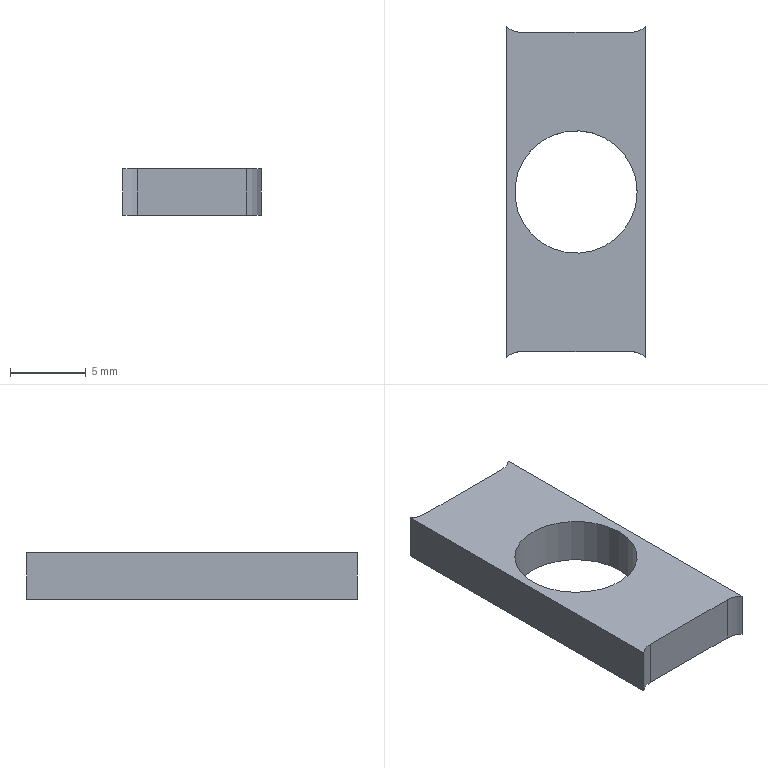Part | STEP file | 1_id370_x_t | 1 solid | 11 faces | box 9.15 x 21.764 x 3.075 mm | volume 435.444 mm3 | plane 6 | cylinder 5 | commonest cylinder face diameters 3 x4 8.06 x1
STEP:
#1=CARTESIAN_POINT('',(0.,0.,0.));
#2=DIRECTION('',(0.,0.,1.));
#3=DIRECTION('',(1.,0.,0.));
#4=AXIS2_PLACEMENT_3D('',#1,#2,#3);
#5=CARTESIAN_POINT('',(383.175,166.618,0.));
#6=VERTEX_POINT('',#5);
#7=CARTESIAN_POINT('',(382.175,167.,0.));
#8=VERTEX_POINT('',#7);
#9=CARTESIAN_POINT('',(382.175,165.5,0.));
#10=DIRECTION('',(0.,0.,1.));
#11=DIRECTION('',(1.,0.,0.));
#12=AXIS2_PLACEMENT_3D('',#9,#10,#11);
#13=CIRCLE('',#12,1.5);
#14=CARTESIAN_POINT('',(382.175,165.5,13.075));
#15=DIRECTION('',(0.,0.,-1.));
#16=DIRECTION('',(-1.,0.,0.));
#17=AXIS2_PLACEMENT_3D('',#14,#15,#16);
#18=CYLINDRICAL_SURFACE('',#17,1.5);
#19=CARTESIAN_POINT('',(3.142,13.075));
#20=DIRECTION('',(-1.,0.));
#21=VECTOR('',#20,1.);
#22=LINE('',#19,#21);
#23=(GEOMETRIC_REPRESENTATION_CONTEXT(2)PARAMETRIC_REPRESENTATION_CONTEXT()REPRESENTATION_CONTEXT('',''));
#24=DEFINITIONAL_REPRESENTATION('',(#22),#23);
#25=PCURVE('',#18,#24);
#26=CARTESIAN_POINT('',(407.126,177.154,0.));
#27=DIRECTION('',(0.,0.,1.));
#28=DIRECTION('',(0.00002249,-1.,0.));
#29=AXIS2_PLACEMENT_3D('',#26,#27,#28);
#30=PLANE('',#29);
#31=CARTESIAN_POINT('',(11.653,-24.951));
#32=DIRECTION('',(0.00002249,1.));
#33=AXIS2_PLACEMENT_2D('',#31,#32);
#34=CIRCLE('',#33,1.5);
#35=(GEOMETRIC_REPRESENTATION_CONTEXT(2)PARAMETRIC_REPRESENTATION_CONTEXT()REPRESENTATION_CONTEXT('',''));
#36=DEFINITIONAL_REPRESENTATION('',(#34),#35);
#37=PCURVE('',#30,#36);
#38=SURFACE_CURVE('',#13,(#25,#37),.PCURVE_S1.);
#39=EDGE_CURVE('',#6,#8,#38,.T.);
#40=ORIENTED_EDGE('',*,*,#39,.T.);
#41=CARTESIAN_POINT('',(382.175,167.,3.075));
#42=VERTEX_POINT('',#41);
#43=CARTESIAN_POINT('',(382.175,167.,13.075));
#44=DIRECTION('',(0.,0.,-1.));
#45=VECTOR('',#44,1.);
#46=LINE('',#43,#45);
#47=CARTESIAN_POINT('',(1.571,0.));
#48=DIRECTION('',(0.,1.));
#49=VECTOR('',#48,1.);
#50=LINE('',#47,#49);
#51=(GEOMETRIC_REPRESENTATION_CONTEXT(2)PARAMETRIC_REPRESENTATION_CONTEXT()REPRESENTATION_CONTEXT('',''));
#52=DEFINITIONAL_REPRESENTATION('',(#50),#51);
#53=PCURVE('',#18,#52);
#54=CARTESIAN_POINT('',(382.175,167.,13.075));
#55=DIRECTION('',(0.,-1.,0.));
#56=DIRECTION('',(0.,0.,-1.));
#57=AXIS2_PLACEMENT_3D('',#54,#55,#56);
#58=PLANE('',#57);
#59=CARTESIAN_POINT('',(0.,0.));
#60=DIRECTION('',(1.,0.));
#61=VECTOR('',#60,1.);
#62=LINE('',#59,#61);
#63=(GEOMETRIC_REPRESENTATION_CONTEXT(2)PARAMETRIC_REPRESENTATION_CONTEXT()REPRESENTATION_CONTEXT('',''));
#64=DEFINITIONAL_REPRESENTATION('',(#62),#63);
#65=PCURVE('',#58,#64);
#66=SURFACE_CURVE('',#46,(#53,#65),.PCURVE_S1.);
#67=EDGE_CURVE('',#42,#8,#66,.T.);
#68=ORIENTED_EDGE('',*,*,#67,.F.);
#69=CARTESIAN_POINT('',(383.175,166.618,3.075));
#70=VERTEX_POINT('',#69);
#71=CARTESIAN_POINT('',(382.175,165.5,3.075));
#72=DIRECTION('',(0.,0.,1.));
#73=DIRECTION('',(1.,0.,0.));
#74=AXIS2_PLACEMENT_3D('',#71,#72,#73);
#75=CIRCLE('',#74,1.5);
#76=CARTESIAN_POINT('',(3.142,10.));
#77=DIRECTION('',(-1.,0.));
#78=VECTOR('',#77,1.);
#79=LINE('',#76,#78);
#80=(GEOMETRIC_REPRESENTATION_CONTEXT(2)PARAMETRIC_REPRESENTATION_CONTEXT()REPRESENTATION_CONTEXT('',''));
#81=DEFINITIONAL_REPRESENTATION('',(#79),#80);
#82=PCURVE('',#18,#81);
#83=CARTESIAN_POINT('',(407.126,177.154,3.075));
#84=DIRECTION('',(0.,0.,1.));
#85=DIRECTION('',(0.00002249,-1.,0.));
#86=AXIS2_PLACEMENT_3D('',#83,#84,#85);
#87=PLANE('',#86);
#88=CARTESIAN_POINT('',(11.653,-24.951));
#89=DIRECTION('',(0.00002249,1.));
#90=AXIS2_PLACEMENT_2D('',#88,#89);
#91=CIRCLE('',#90,1.5);
#92=(GEOMETRIC_REPRESENTATION_CONTEXT(2)PARAMETRIC_REPRESENTATION_CONTEXT()REPRESENTATION_CONTEXT('',''));
#93=DEFINITIONAL_REPRESENTATION('',(#91),#92);
#94=PCURVE('',#87,#93);
#95=SURFACE_CURVE('',#75,(#82,#94),.PCURVE_S1.);
#96=EDGE_CURVE('',#70,#42,#95,.T.);
#97=ORIENTED_EDGE('',*,*,#96,.F.);
#98=CARTESIAN_POINT('',(383.175,166.618,13.075));
#99=DIRECTION('',(0.,0.,-1.));
#100=VECTOR('',#99,1.);
#101=LINE('',#98,#100);
#102=CARTESIAN_POINT('',(2.301,0.));
#103=DIRECTION('',(0.,1.));
#104=VECTOR('',#103,1.);
#105=LINE('',#102,#104);
#106=(GEOMETRIC_REPRESENTATION_CONTEXT(2)PARAMETRIC_REPRESENTATION_CONTEXT()REPRESENTATION_CONTEXT('',''));
#107=DEFINITIONAL_REPRESENTATION('',(#105),#106);
#108=PCURVE('',#18,#107);
#109=CARTESIAN_POINT('',(383.175,183.602,7.112));
#110=DIRECTION('',(-1.,0.,0.));
#111=DIRECTION('',(0.,0.,1.));
#112=AXIS2_PLACEMENT_3D('',#109,#110,#111);
#113=PLANE('',#112);
#114=CARTESIAN_POINT('',(5.962,-16.984));
#115=DIRECTION('',(-1.,0.));
#116=VECTOR('',#115,1.);
#117=LINE('',#114,#116);
#118=(GEOMETRIC_REPRESENTATION_CONTEXT(2)PARAMETRIC_REPRESENTATION_CONTEXT()REPRESENTATION_CONTEXT('',''));
#119=DEFINITIONAL_REPRESENTATION('',(#117),#118);
#120=PCURVE('',#113,#119);
#121=SURFACE_CURVE('',#101,(#108,#120),.PCURVE_S1.);
#122=EDGE_CURVE('',#70,#6,#121,.T.);
#123=ORIENTED_EDGE('',*,*,#122,.T.);
#124=EDGE_LOOP('',(#40,#68,#97,#123));
#125=FACE_BOUND('',#124,.F.);
#126=ADVANCED_FACE('',(#125),#18,.F.);
#127=CARTESIAN_POINT('',(383.175,188.382,0.));
#128=VERTEX_POINT('',#127);
#129=CARTESIAN_POINT('',(383.175,177.154,0.));
#130=DIRECTION('',(0.,1.,0.));
#131=VECTOR('',#130,1.);
#132=LINE('',#129,#131);
#133=CARTESIAN_POINT('',(-7.112,-6.448));
#134=DIRECTION('',(0.,1.));
#135=VECTOR('',#134,1.);
#136=LINE('',#133,#135);
#137=(GEOMETRIC_REPRESENTATION_CONTEXT(2)PARAMETRIC_REPRESENTATION_CONTEXT()REPRESENTATION_CONTEXT('',''));
#138=DEFINITIONAL_REPRESENTATION('',(#136),#137);
#139=PCURVE('',#113,#138);
#140=CARTESIAN_POINT('',(-0.0005386,-23.951));
#141=DIRECTION('',(-1.,0.00002249));
#142=VECTOR('',#141,1.);
#143=LINE('',#140,#142);
#144=(GEOMETRIC_REPRESENTATION_CONTEXT(2)PARAMETRIC_REPRESENTATION_CONTEXT()REPRESENTATION_CONTEXT('',''));
#145=DEFINITIONAL_REPRESENTATION('',(#143),#144);
#146=PCURVE('',#30,#145);
#147=SURFACE_CURVE('',#132,(#139,#146),.PCURVE_S1.);
#148=EDGE_CURVE('',#6,#128,#147,.T.);
#149=ORIENTED_EDGE('',*,*,#148,.T.);
#150=CARTESIAN_POINT('',(383.175,188.382,3.075));
#151=VERTEX_POINT('',#150);
#152=CARTESIAN_POINT('',(383.175,188.382,13.075));
#153=DIRECTION('',(0.,0.,-1.));
#154=VECTOR('',#153,1.);
#155=LINE('',#152,#154);
#156=CARTESIAN_POINT('',(5.962,4.78));
#157=DIRECTION('',(-1.,0.));
#158=VECTOR('',#157,1.);
#159=LINE('',#156,#158);
#160=(GEOMETRIC_REPRESENTATION_CONTEXT(2)PARAMETRIC_REPRESENTATION_CONTEXT()REPRESENTATION_CONTEXT('',''));
#161=DEFINITIONAL_REPRESENTATION('',(#159),#160);
#162=PCURVE('',#113,#161);
#163=CARTESIAN_POINT('',(382.175,189.5,13.075));
#164=DIRECTION('',(0.,0.,-1.));
#165=DIRECTION('',(-1.,0.,0.));
#166=AXIS2_PLACEMENT_3D('',#163,#164,#165);
#167=CYLINDRICAL_SURFACE('',#166,1.5);
#168=CARTESIAN_POINT('',(3.983,0.));
#169=DIRECTION('',(0.,1.));
#170=VECTOR('',#169,1.);
#171=LINE('',#168,#170);
#172=(GEOMETRIC_REPRESENTATION_CONTEXT(2)PARAMETRIC_REPRESENTATION_CONTEXT()REPRESENTATION_CONTEXT('',''));
#173=DEFINITIONAL_REPRESENTATION('',(#171),#172);
#174=PCURVE('',#167,#173);
#175=SURFACE_CURVE('',#155,(#162,#174),.PCURVE_S1.);
#176=EDGE_CURVE('',#151,#128,#175,.T.);
#177=ORIENTED_EDGE('',*,*,#176,.F.);
#178=CARTESIAN_POINT('',(383.175,177.154,3.075));
#179=DIRECTION('',(0.,1.,0.));
#180=VECTOR('',#179,1.);
#181=LINE('',#178,#180);
#182=CARTESIAN_POINT('',(-4.037,-6.448));
#183=DIRECTION('',(0.,1.));
#184=VECTOR('',#183,1.);
#185=LINE('',#182,#184);
#186=(GEOMETRIC_REPRESENTATION_CONTEXT(2)PARAMETRIC_REPRESENTATION_CONTEXT()REPRESENTATION_CONTEXT('',''));
#187=DEFINITIONAL_REPRESENTATION('',(#185),#186);
#188=PCURVE('',#113,#187);
#189=CARTESIAN_POINT('',(-0.0005386,-23.951));
#190=DIRECTION('',(-1.,0.00002249));
#191=VECTOR('',#190,1.);
#192=LINE('',#189,#191);
#193=(GEOMETRIC_REPRESENTATION_CONTEXT(2)PARAMETRIC_REPRESENTATION_CONTEXT()REPRESENTATION_CONTEXT('',''));
#194=DEFINITIONAL_REPRESENTATION('',(#192),#193);
#195=PCURVE('',#87,#194);
#196=SURFACE_CURVE('',#181,(#188,#195),.PCURVE_S1.);
#197=EDGE_CURVE('',#70,#151,#196,.T.);
#198=ORIENTED_EDGE('',*,*,#197,.F.);
#199=ORIENTED_EDGE('',*,*,#122,.T.);
#200=EDGE_LOOP('',(#149,#177,#198,#199));
#201=FACE_BOUND('',#200,.T.);
#202=ADVANCED_FACE('',(#201),#113,.F.);
#203=CARTESIAN_POINT('',(375.025,167.,3.075));
#204=VERTEX_POINT('',#203);
#205=CARTESIAN_POINT('',(407.126,167.,3.075));
#206=DIRECTION('',(-1.,0.,0.));
#207=VECTOR('',#206,1.);
#208=LINE('',#205,#207);
#209=CARTESIAN_POINT('',(10.,24.951));
#210=DIRECTION('',(0.,-1.));
#211=VECTOR('',#210,1.);
#212=LINE('',#209,#211);
#213=(GEOMETRIC_REPRESENTATION_CONTEXT(2)PARAMETRIC_REPRESENTATION_CONTEXT()REPRESENTATION_CONTEXT('',''));
#214=DEFINITIONAL_REPRESENTATION('',(#212),#213);
#215=PCURVE('',#58,#214);
#216=CARTESIAN_POINT('',(10.154,-0.0002283));
#217=DIRECTION('',(-0.00002249,-1.));
#218=VECTOR('',#217,1.);
#219=LINE('',#216,#218);
#220=(GEOMETRIC_REPRESENTATION_CONTEXT(2)PARAMETRIC_REPRESENTATION_CONTEXT()REPRESENTATION_CONTEXT('',''));
#221=DEFINITIONAL_REPRESENTATION('',(#219),#220);
#222=PCURVE('',#87,#221);
#223=SURFACE_CURVE('',#208,(#215,#222),.PCURVE_S1.);
#224=EDGE_CURVE('',#42,#204,#223,.T.);
#225=ORIENTED_EDGE('',*,*,#224,.T.);
#226=CARTESIAN_POINT('',(375.025,167.,0.));
#227=VERTEX_POINT('',#226);
#228=CARTESIAN_POINT('',(375.025,167.,13.075));
#229=DIRECTION('',(0.,0.,-1.));
#230=VECTOR('',#229,1.);
#231=LINE('',#228,#230);
#232=CARTESIAN_POINT('',(0.,-7.15));
#233=DIRECTION('',(1.,0.));
#234=VECTOR('',#233,1.);
#235=LINE('',#232,#234);
#236=(GEOMETRIC_REPRESENTATION_CONTEXT(2)PARAMETRIC_REPRESENTATION_CONTEXT()REPRESENTATION_CONTEXT('',''));
#237=DEFINITIONAL_REPRESENTATION('',(#235),#236);
#238=PCURVE('',#58,#237);
#239=CARTESIAN_POINT('',(375.025,165.5,13.075));
#240=DIRECTION('',(0.,0.,-1.));
#241=DIRECTION('',(-1.,0.,0.));
#242=AXIS2_PLACEMENT_3D('',#239,#240,#241);
#243=CYLINDRICAL_SURFACE('',#242,1.5);
#244=CARTESIAN_POINT('',(1.571,0.));
#245=DIRECTION('',(0.,1.));
#246=VECTOR('',#245,1.);
#247=LINE('',#244,#246);
#248=(GEOMETRIC_REPRESENTATION_CONTEXT(2)PARAMETRIC_REPRESENTATION_CONTEXT()REPRESENTATION_CONTEXT('',''));
#249=DEFINITIONAL_REPRESENTATION('',(#247),#248);
#250=PCURVE('',#243,#249);
#251=SURFACE_CURVE('',#231,(#238,#250),.PCURVE_S1.);
#252=EDGE_CURVE('',#204,#227,#251,.T.);
#253=ORIENTED_EDGE('',*,*,#252,.T.);
#254=CARTESIAN_POINT('',(407.126,167.,0.));
#255=DIRECTION('',(-1.,0.,0.));
#256=VECTOR('',#255,1.);
#257=LINE('',#254,#256);
#258=CARTESIAN_POINT('',(13.075,24.951));
#259=DIRECTION('',(0.,-1.));
#260=VECTOR('',#259,1.);
#261=LINE('',#258,#260);
#262=(GEOMETRIC_REPRESENTATION_CONTEXT(2)PARAMETRIC_REPRESENTATION_CONTEXT()REPRESENTATION_CONTEXT('',''));
#263=DEFINITIONAL_REPRESENTATION('',(#261),#262);
#264=PCURVE('',#58,#263);
#265=CARTESIAN_POINT('',(10.154,-0.0002283));
#266=DIRECTION('',(-0.00002249,-1.));
#267=VECTOR('',#266,1.);
#268=LINE('',#265,#267);
#269=(GEOMETRIC_REPRESENTATION_CONTEXT(2)PARAMETRIC_REPRESENTATION_CONTEXT()REPRESENTATION_CONTEXT('',''));
#270=DEFINITIONAL_REPRESENTATION('',(#268),#269);
#271=PCURVE('',#30,#270);
#272=SURFACE_CURVE('',#257,(#264,#271),.PCURVE_S1.);
#273=EDGE_CURVE('',#8,#227,#272,.T.);
#274=ORIENTED_EDGE('',*,*,#273,.F.);
#275=ORIENTED_EDGE('',*,*,#67,.F.);
#276=EDGE_LOOP('',(#225,#253,#274,#275));
#277=FACE_BOUND('',#276,.T.);
#278=ADVANCED_FACE('',(#277),#58,.T.);
#279=ORIENTED_EDGE('',*,*,#252,.T.);
#280=CARTESIAN_POINT('',(374.025,166.618,0.));
#281=VERTEX_POINT('',#280);
#282=CARTESIAN_POINT('',(375.025,165.5,0.));
#283=DIRECTION('',(0.,0.,1.));
#284=DIRECTION('',(1.,0.,0.));
#285=AXIS2_PLACEMENT_3D('',#282,#283,#284);
#286=CIRCLE('',#285,1.5);
#287=CARTESIAN_POINT('',(3.142,13.075));
#288=DIRECTION('',(-1.,0.));
#289=VECTOR('',#288,1.);
#290=LINE('',#287,#289);
#291=(GEOMETRIC_REPRESENTATION_CONTEXT(2)PARAMETRIC_REPRESENTATION_CONTEXT()REPRESENTATION_CONTEXT('',''));
#292=DEFINITIONAL_REPRESENTATION('',(#290),#291);
#293=PCURVE('',#243,#292);
#294=CARTESIAN_POINT('',(11.653,-32.101));
#295=DIRECTION('',(0.00002249,1.));
#296=AXIS2_PLACEMENT_2D('',#294,#295);
#297=CIRCLE('',#296,1.5);
#298=(GEOMETRIC_REPRESENTATION_CONTEXT(2)PARAMETRIC_REPRESENTATION_CONTEXT()REPRESENTATION_CONTEXT('',''));
#299=DEFINITIONAL_REPRESENTATION('',(#297),#298);
#300=PCURVE('',#30,#299);
#301=SURFACE_CURVE('',#286,(#293,#300),.PCURVE_S1.);
#302=EDGE_CURVE('',#227,#281,#301,.T.);
#303=ORIENTED_EDGE('',*,*,#302,.T.);
#304=CARTESIAN_POINT('',(374.025,166.618,3.075));
#305=VERTEX_POINT('',#304);
#306=CARTESIAN_POINT('',(374.025,166.618,13.075));
#307=DIRECTION('',(0.,0.,-1.));
#308=VECTOR('',#307,1.);
#309=LINE('',#306,#308);
#310=CARTESIAN_POINT('',(0.8411,0.));
#311=DIRECTION('',(0.,1.));
#312=VECTOR('',#311,1.);
#313=LINE('',#310,#312);
#314=(GEOMETRIC_REPRESENTATION_CONTEXT(2)PARAMETRIC_REPRESENTATION_CONTEXT()REPRESENTATION_CONTEXT('',''));
#315=DEFINITIONAL_REPRESENTATION('',(#313),#314);
#316=PCURVE('',#243,#315);
#317=CARTESIAN_POINT('',(374.025,183.602,7.112));
#318=DIRECTION('',(-1.,0.,0.));
#319=DIRECTION('',(0.,0.,1.));
#320=AXIS2_PLACEMENT_3D('',#317,#318,#319);
#321=PLANE('',#320);
#322=CARTESIAN_POINT('',(5.962,-16.984));
#323=DIRECTION('',(-1.,0.));
#324=VECTOR('',#323,1.);
#325=LINE('',#322,#324);
#326=(GEOMETRIC_REPRESENTATION_CONTEXT(2)PARAMETRIC_REPRESENTATION_CONTEXT()REPRESENTATION_CONTEXT('',''));
#327=DEFINITIONAL_REPRESENTATION('',(#325),#326);
#328=PCURVE('',#321,#327);
#329=SURFACE_CURVE('',#309,(#316,#328),.PCURVE_S1.);
#330=EDGE_CURVE('',#305,#281,#329,.T.);
#331=ORIENTED_EDGE('',*,*,#330,.F.);
#332=CARTESIAN_POINT('',(375.025,165.5,3.075));
#333=DIRECTION('',(0.,0.,1.));
#334=DIRECTION('',(1.,0.,0.));
#335=AXIS2_PLACEMENT_3D('',#332,#333,#334);
#336=CIRCLE('',#335,1.5);
#337=CARTESIAN_POINT('',(3.142,10.));
#338=DIRECTION('',(-1.,0.));
#339=VECTOR('',#338,1.);
#340=LINE('',#337,#339);
#341=(GEOMETRIC_REPRESENTATION_CONTEXT(2)PARAMETRIC_REPRESENTATION_CONTEXT()REPRESENTATION_CONTEXT('',''));
#342=DEFINITIONAL_REPRESENTATION('',(#340),#341);
#343=PCURVE('',#243,#342);
#344=CARTESIAN_POINT('',(11.653,-32.101));
#345=DIRECTION('',(0.00002249,1.));
#346=AXIS2_PLACEMENT_2D('',#344,#345);
#347=CIRCLE('',#346,1.5);
#348=(GEOMETRIC_REPRESENTATION_CONTEXT(2)PARAMETRIC_REPRESENTATION_CONTEXT()REPRESENTATION_CONTEXT('',''));
#349=DEFINITIONAL_REPRESENTATION('',(#347),#348);
#350=PCURVE('',#87,#349);
#351=SURFACE_CURVE('',#336,(#343,#350),.PCURVE_S1.);
#352=EDGE_CURVE('',#204,#305,#351,.T.);
#353=ORIENTED_EDGE('',*,*,#352,.F.);
#354=EDGE_LOOP('',(#279,#303,#331,#353));
#355=FACE_BOUND('',#354,.F.);
#356=ADVANCED_FACE('',(#355),#243,.F.);
#357=CARTESIAN_POINT('',(382.63,177.5,0.));
#358=VERTEX_POINT('',#357);
#359=CARTESIAN_POINT('',(378.6,177.5,0.));
#360=DIRECTION('',(0.,0.,-1.));
#361=DIRECTION('',(1.,0.,0.));
#362=AXIS2_PLACEMENT_3D('',#359,#360,#361);
#363=CIRCLE('',#362,4.03);
#364=CARTESIAN_POINT('',(-0.3469,-24.496));
#365=CARTESIAN_POINT('',(6.633,-24.496));
#366=CARTESIAN_POINT('',(3.143,-30.541));
#367=CARTESIAN_POINT('',(-0.3472,-36.586));
#368=CARTESIAN_POINT('',(-3.837,-30.541));
#369=CARTESIAN_POINT('',(-7.327,-24.496));
#370=CARTESIAN_POINT('',(-0.3469,-24.496));
#371=(BOUNDED_CURVE()B_SPLINE_CURVE(2,(#364,#365,#366,#367,#368,#369,#370),.UNSPECIFIED.,.T.,.F.)B_SPLINE_CURVE_WITH_KNOTS((1,2,2,2,2,1),(-2.094,0.,2.094,4.189,6.283,8.378),.UNSPECIFIED.)CURVE()GEOMETRIC_REPRESENTATION_ITEM()RATIONAL_B_SPLINE_CURVE((1.,0.5,1.,0.5,1.,0.5,1.))REPRESENTATION_ITEM(''));
#372=(GEOMETRIC_REPRESENTATION_CONTEXT(2)PARAMETRIC_REPRESENTATION_CONTEXT()REPRESENTATION_CONTEXT('',''));
#373=DEFINITIONAL_REPRESENTATION('',(#371),#372);
#374=PCURVE('',#30,#373);
#375=CARTESIAN_POINT('',(378.6,177.5,10.));
#376=DIRECTION('',(0.,0.,-1.));
#377=DIRECTION('',(-1.,0.,0.));
#378=AXIS2_PLACEMENT_3D('',#375,#376,#377);
#379=CYLINDRICAL_SURFACE('',#378,4.03);
#380=CARTESIAN_POINT('',(3.142,10.));
#381=DIRECTION('',(1.,0.));
#382=VECTOR('',#381,1.);
#383=LINE('',#380,#382);
#384=(GEOMETRIC_REPRESENTATION_CONTEXT(2)PARAMETRIC_REPRESENTATION_CONTEXT()REPRESENTATION_CONTEXT('',''));
#385=DEFINITIONAL_REPRESENTATION('',(#383),#384);
#386=PCURVE('',#379,#385);
#387=SURFACE_CURVE('',#363,(#374,#386),.PCURVE_S1.);
#388=EDGE_CURVE('',#358,#358,#387,.T.);
#389=ORIENTED_EDGE('',*,*,#388,.F.);
#390=EDGE_LOOP('',(#389));
#391=FACE_BOUND('',#390,.T.);
#392=CARTESIAN_POINT('',(382.175,188.,0.));
#393=VERTEX_POINT('',#392);
#394=CARTESIAN_POINT('',(382.175,189.5,0.));
#395=DIRECTION('',(0.,0.,-1.));
#396=DIRECTION('',(1.,0.,0.));
#397=AXIS2_PLACEMENT_3D('',#394,#395,#396);
#398=CIRCLE('',#397,1.5);
#399=CARTESIAN_POINT('',(-12.347,-23.451));
#400=CARTESIAN_POINT('',(-9.749,-23.451));
#401=CARTESIAN_POINT('',(-11.048,-25.701));
#402=CARTESIAN_POINT('',(-12.347,-27.951));
#403=CARTESIAN_POINT('',(-13.646,-25.701));
#404=CARTESIAN_POINT('',(-14.945,-23.451));
#405=CARTESIAN_POINT('',(-12.347,-23.451));
#406=(BOUNDED_CURVE()B_SPLINE_CURVE(2,(#399,#400,#401,#402,#403,#404,#405),.UNSPECIFIED.,.T.,.F.)B_SPLINE_CURVE_WITH_KNOTS((1,2,2,2,2,1),(-2.094,0.,2.094,4.189,6.283,8.378),.UNSPECIFIED.)CURVE()GEOMETRIC_REPRESENTATION_ITEM()RATIONAL_B_SPLINE_CURVE((1.,0.5,1.,0.5,1.,0.5,1.))REPRESENTATION_ITEM(''));
#407=(GEOMETRIC_REPRESENTATION_CONTEXT(2)PARAMETRIC_REPRESENTATION_CONTEXT()REPRESENTATION_CONTEXT('',''));
#408=DEFINITIONAL_REPRESENTATION('',(#406),#407);
#409=PCURVE('',#30,#408);
#410=CARTESIAN_POINT('',(3.142,13.075));
#411=DIRECTION('',(1.,0.));
#412=VECTOR('',#411,1.);
#413=LINE('',#410,#412);
#414=(GEOMETRIC_REPRESENTATION_CONTEXT(2)PARAMETRIC_REPRESENTATION_CONTEXT()REPRESENTATION_CONTEXT('',''));
#415=DEFINITIONAL_REPRESENTATION('',(#413),#414);
#416=PCURVE('',#167,#415);
#417=SURFACE_CURVE('',#398,(#409,#416),.PCURVE_S1.);
#418=EDGE_CURVE('',#128,#393,#417,.T.);
#419=ORIENTED_EDGE('',*,*,#418,.F.);
#420=ORIENTED_EDGE('',*,*,#148,.F.);
#421=ORIENTED_EDGE('',*,*,#39,.T.);
#422=ORIENTED_EDGE('',*,*,#273,.T.);
#423=ORIENTED_EDGE('',*,*,#302,.T.);
#424=CARTESIAN_POINT('',(374.025,188.382,0.));
#425=VERTEX_POINT('',#424);
#426=CARTESIAN_POINT('',(374.025,177.154,0.));
#427=DIRECTION('',(0.,1.,0.));
#428=VECTOR('',#427,1.);
#429=LINE('',#426,#428);
#430=CARTESIAN_POINT('',(-0.0007443,-33.101));
#431=DIRECTION('',(-1.,0.00002249));
#432=VECTOR('',#431,1.);
#433=LINE('',#430,#432);
#434=(GEOMETRIC_REPRESENTATION_CONTEXT(2)PARAMETRIC_REPRESENTATION_CONTEXT()REPRESENTATION_CONTEXT('',''));
#435=DEFINITIONAL_REPRESENTATION('',(#433),#434);
#436=PCURVE('',#30,#435);
#437=CARTESIAN_POINT('',(-7.112,-6.448));
#438=DIRECTION('',(0.,1.));
#439=VECTOR('',#438,1.);
#440=LINE('',#437,#439);
#441=(GEOMETRIC_REPRESENTATION_CONTEXT(2)PARAMETRIC_REPRESENTATION_CONTEXT()REPRESENTATION_CONTEXT('',''));
#442=DEFINITIONAL_REPRESENTATION('',(#440),#441);
#443=PCURVE('',#321,#442);
#444=SURFACE_CURVE('',#429,(#436,#443),.PCURVE_S1.);
#445=EDGE_CURVE('',#281,#425,#444,.T.);
#446=ORIENTED_EDGE('',*,*,#445,.T.);
#447=CARTESIAN_POINT('',(375.025,188.,0.));
#448=VERTEX_POINT('',#447);
#449=CARTESIAN_POINT('',(375.025,189.5,0.));
#450=DIRECTION('',(0.,0.,-1.));
#451=DIRECTION('',(1.,0.,0.));
#452=AXIS2_PLACEMENT_3D('',#449,#450,#451);
#453=CIRCLE('',#452,1.5);
#454=CARTESIAN_POINT('',(-12.347,-30.601));
#455=CARTESIAN_POINT('',(-9.749,-30.601));
#456=CARTESIAN_POINT('',(-11.048,-32.851));
#457=CARTESIAN_POINT('',(-12.347,-35.101));
#458=CARTESIAN_POINT('',(-13.646,-32.851));
#459=CARTESIAN_POINT('',(-14.945,-30.601));
#460=CARTESIAN_POINT('',(-12.347,-30.601));
#461=(BOUNDED_CURVE()B_SPLINE_CURVE(2,(#454,#455,#456,#457,#458,#459,#460),.UNSPECIFIED.,.T.,.F.)B_SPLINE_CURVE_WITH_KNOTS((1,2,2,2,2,1),(-2.094,0.,2.094,4.189,6.283,8.378),.UNSPECIFIED.)CURVE()GEOMETRIC_REPRESENTATION_ITEM()RATIONAL_B_SPLINE_CURVE((1.,0.5,1.,0.5,1.,0.5,1.))REPRESENTATION_ITEM(''));
#462=(GEOMETRIC_REPRESENTATION_CONTEXT(2)PARAMETRIC_REPRESENTATION_CONTEXT()REPRESENTATION_CONTEXT('',''));
#463=DEFINITIONAL_REPRESENTATION('',(#461),#462);
#464=PCURVE('',#30,#463);
#465=CARTESIAN_POINT('',(375.025,189.5,13.075));
#466=DIRECTION('',(0.,0.,-1.));
#467=DIRECTION('',(-1.,0.,0.));
#468=AXIS2_PLACEMENT_3D('',#465,#466,#467);
#469=CYLINDRICAL_SURFACE('',#468,1.5);
#470=CARTESIAN_POINT('',(3.142,13.075));
#471=DIRECTION('',(1.,0.));
#472=VECTOR('',#471,1.);
#473=LINE('',#470,#472);
#474=(GEOMETRIC_REPRESENTATION_CONTEXT(2)PARAMETRIC_REPRESENTATION_CONTEXT()REPRESENTATION_CONTEXT('',''));
#475=DEFINITIONAL_REPRESENTATION('',(#473),#474);
#476=PCURVE('',#469,#475);
#477=SURFACE_CURVE('',#453,(#464,#476),.PCURVE_S1.);
#478=EDGE_CURVE('',#448,#425,#477,.T.);
#479=ORIENTED_EDGE('',*,*,#478,.F.);
#480=CARTESIAN_POINT('',(407.126,188.,0.));
#481=DIRECTION('',(-1.,0.,0.));
#482=VECTOR('',#481,1.);
#483=LINE('',#480,#482);
#484=CARTESIAN_POINT('',(-10.846,0.0002439));
#485=DIRECTION('',(-0.00002249,-1.));
#486=VECTOR('',#485,1.);
#487=LINE('',#484,#486);
#488=(GEOMETRIC_REPRESENTATION_CONTEXT(2)PARAMETRIC_REPRESENTATION_CONTEXT()REPRESENTATION_CONTEXT('',''));
#489=DEFINITIONAL_REPRESENTATION('',(#487),#488);
#490=PCURVE('',#30,#489);
#491=CARTESIAN_POINT('',(382.175,188.,13.075));
#492=DIRECTION('',(0.,-1.,0.));
#493=DIRECTION('',(0.,0.,-1.));
#494=AXIS2_PLACEMENT_3D('',#491,#492,#493);
#495=PLANE('',#494);
#496=CARTESIAN_POINT('',(13.075,24.951));
#497=DIRECTION('',(0.,-1.));
#498=VECTOR('',#497,1.);
#499=LINE('',#496,#498);
#500=(GEOMETRIC_REPRESENTATION_CONTEXT(2)PARAMETRIC_REPRESENTATION_CONTEXT()REPRESENTATION_CONTEXT('',''));
#501=DEFINITIONAL_REPRESENTATION('',(#499),#500);
#502=PCURVE('',#495,#501);
#503=SURFACE_CURVE('',#483,(#490,#502),.PCURVE_S1.);
#504=EDGE_CURVE('',#393,#448,#503,.T.);
#505=ORIENTED_EDGE('',*,*,#504,.F.);
#506=EDGE_LOOP('',(#419,#420,#421,#422,#423,#446,#479,#505));
#507=FACE_BOUND('',#506,.T.);
#508=ADVANCED_FACE('',(#391,#507),#30,.F.);
#509=CARTESIAN_POINT('',(382.63,177.5,3.075));
#510=VERTEX_POINT('',#509);
#511=CARTESIAN_POINT('',(378.6,177.5,3.075));
#512=DIRECTION('',(0.,0.,-1.));
#513=DIRECTION('',(1.,0.,0.));
#514=AXIS2_PLACEMENT_3D('',#511,#512,#513);
#515=CIRCLE('',#514,4.03);
#516=CARTESIAN_POINT('',(-0.3469,-24.496));
#517=CARTESIAN_POINT('',(6.633,-24.496));
#518=CARTESIAN_POINT('',(3.143,-30.541));
#519=CARTESIAN_POINT('',(-0.3472,-36.586));
#520=CARTESIAN_POINT('',(-3.837,-30.541));
#521=CARTESIAN_POINT('',(-7.327,-24.496));
#522=CARTESIAN_POINT('',(-0.3469,-24.496));
#523=(BOUNDED_CURVE()B_SPLINE_CURVE(2,(#516,#517,#518,#519,#520,#521,#522),.UNSPECIFIED.,.T.,.F.)B_SPLINE_CURVE_WITH_KNOTS((1,2,2,2,2,1),(-2.094,0.,2.094,4.189,6.283,8.378),.UNSPECIFIED.)CURVE()GEOMETRIC_REPRESENTATION_ITEM()RATIONAL_B_SPLINE_CURVE((1.,0.5,1.,0.5,1.,0.5,1.))REPRESENTATION_ITEM(''));
#524=(GEOMETRIC_REPRESENTATION_CONTEXT(2)PARAMETRIC_REPRESENTATION_CONTEXT()REPRESENTATION_CONTEXT('',''));
#525=DEFINITIONAL_REPRESENTATION('',(#523),#524);
#526=PCURVE('',#87,#525);
#527=CARTESIAN_POINT('',(3.142,6.925));
#528=DIRECTION('',(1.,0.));
#529=VECTOR('',#528,1.);
#530=LINE('',#527,#529);
#531=(GEOMETRIC_REPRESENTATION_CONTEXT(2)PARAMETRIC_REPRESENTATION_CONTEXT()REPRESENTATION_CONTEXT('',''));
#532=DEFINITIONAL_REPRESENTATION('',(#530),#531);
#533=PCURVE('',#379,#532);
#534=SURFACE_CURVE('',#515,(#526,#533),.PCURVE_S1.);
#535=EDGE_CURVE('',#510,#510,#534,.T.);
#536=ORIENTED_EDGE('',*,*,#535,.T.);
#537=EDGE_LOOP('',(#536));
#538=FACE_BOUND('',#537,.T.);
#539=ORIENTED_EDGE('',*,*,#197,.T.);
#540=CARTESIAN_POINT('',(382.175,188.,3.075));
#541=VERTEX_POINT('',#540);
#542=CARTESIAN_POINT('',(382.175,189.5,3.075));
#543=DIRECTION('',(0.,0.,-1.));
#544=DIRECTION('',(1.,0.,0.));
#545=AXIS2_PLACEMENT_3D('',#542,#543,#544);
#546=CIRCLE('',#545,1.5);
#547=CARTESIAN_POINT('',(-12.347,-23.451));
#548=CARTESIAN_POINT('',(-9.749,-23.451));
#549=CARTESIAN_POINT('',(-11.048,-25.701));
#550=CARTESIAN_POINT('',(-12.347,-27.951));
#551=CARTESIAN_POINT('',(-13.646,-25.701));
#552=CARTESIAN_POINT('',(-14.945,-23.451));
#553=CARTESIAN_POINT('',(-12.347,-23.451));
#554=(BOUNDED_CURVE()B_SPLINE_CURVE(2,(#547,#548,#549,#550,#551,#552,#553),.UNSPECIFIED.,.T.,.F.)B_SPLINE_CURVE_WITH_KNOTS((1,2,2,2,2,1),(-2.094,0.,2.094,4.189,6.283,8.378),.UNSPECIFIED.)CURVE()GEOMETRIC_REPRESENTATION_ITEM()RATIONAL_B_SPLINE_CURVE((1.,0.5,1.,0.5,1.,0.5,1.))REPRESENTATION_ITEM(''));
#555=(GEOMETRIC_REPRESENTATION_CONTEXT(2)PARAMETRIC_REPRESENTATION_CONTEXT()REPRESENTATION_CONTEXT('',''));
#556=DEFINITIONAL_REPRESENTATION('',(#554),#555);
#557=PCURVE('',#87,#556);
#558=CARTESIAN_POINT('',(3.142,10.));
#559=DIRECTION('',(1.,0.));
#560=VECTOR('',#559,1.);
#561=LINE('',#558,#560);
#562=(GEOMETRIC_REPRESENTATION_CONTEXT(2)PARAMETRIC_REPRESENTATION_CONTEXT()REPRESENTATION_CONTEXT('',''));
#563=DEFINITIONAL_REPRESENTATION('',(#561),#562);
#564=PCURVE('',#167,#563);
#565=SURFACE_CURVE('',#546,(#557,#564),.PCURVE_S1.);
#566=EDGE_CURVE('',#151,#541,#565,.T.);
#567=ORIENTED_EDGE('',*,*,#566,.T.);
#568=CARTESIAN_POINT('',(375.025,188.,3.075));
#569=VERTEX_POINT('',#568);
#570=CARTESIAN_POINT('',(407.126,188.,3.075));
#571=DIRECTION('',(-1.,0.,0.));
#572=VECTOR('',#571,1.);
#573=LINE('',#570,#572);
#574=CARTESIAN_POINT('',(-10.846,0.0002439));
#575=DIRECTION('',(-0.00002249,-1.));
#576=VECTOR('',#575,1.);
#577=LINE('',#574,#576);
#578=(GEOMETRIC_REPRESENTATION_CONTEXT(2)PARAMETRIC_REPRESENTATION_CONTEXT()REPRESENTATION_CONTEXT('',''));
#579=DEFINITIONAL_REPRESENTATION('',(#577),#578);
#580=PCURVE('',#87,#579);
#581=CARTESIAN_POINT('',(10.,24.951));
#582=DIRECTION('',(0.,-1.));
#583=VECTOR('',#582,1.);
#584=LINE('',#581,#583);
#585=(GEOMETRIC_REPRESENTATION_CONTEXT(2)PARAMETRIC_REPRESENTATION_CONTEXT()REPRESENTATION_CONTEXT('',''));
#586=DEFINITIONAL_REPRESENTATION('',(#584),#585);
#587=PCURVE('',#495,#586);
#588=SURFACE_CURVE('',#573,(#580,#587),.PCURVE_S1.);
#589=EDGE_CURVE('',#541,#569,#588,.T.);
#590=ORIENTED_EDGE('',*,*,#589,.T.);
#591=CARTESIAN_POINT('',(374.025,188.382,3.075));
#592=VERTEX_POINT('',#591);
#593=CARTESIAN_POINT('',(375.025,189.5,3.075));
#594=DIRECTION('',(0.,0.,-1.));
#595=DIRECTION('',(1.,0.,0.));
#596=AXIS2_PLACEMENT_3D('',#593,#594,#595);
#597=CIRCLE('',#596,1.5);
#598=CARTESIAN_POINT('',(-12.347,-30.601));
#599=CARTESIAN_POINT('',(-9.749,-30.601));
#600=CARTESIAN_POINT('',(-11.048,-32.851));
#601=CARTESIAN_POINT('',(-12.347,-35.101));
#602=CARTESIAN_POINT('',(-13.646,-32.851));
#603=CARTESIAN_POINT('',(-14.945,-30.601));
#604=CARTESIAN_POINT('',(-12.347,-30.601));
#605=(BOUNDED_CURVE()B_SPLINE_CURVE(2,(#598,#599,#600,#601,#602,#603,#604),.UNSPECIFIED.,.T.,.F.)B_SPLINE_CURVE_WITH_KNOTS((1,2,2,2,2,1),(-2.094,0.,2.094,4.189,6.283,8.378),.UNSPECIFIED.)CURVE()GEOMETRIC_REPRESENTATION_ITEM()RATIONAL_B_SPLINE_CURVE((1.,0.5,1.,0.5,1.,0.5,1.))REPRESENTATION_ITEM(''));
#606=(GEOMETRIC_REPRESENTATION_CONTEXT(2)PARAMETRIC_REPRESENTATION_CONTEXT()REPRESENTATION_CONTEXT('',''));
#607=DEFINITIONAL_REPRESENTATION('',(#605),#606);
#608=PCURVE('',#87,#607);
#609=CARTESIAN_POINT('',(3.142,10.));
#610=DIRECTION('',(1.,0.));
#611=VECTOR('',#610,1.);
#612=LINE('',#609,#611);
#613=(GEOMETRIC_REPRESENTATION_CONTEXT(2)PARAMETRIC_REPRESENTATION_CONTEXT()REPRESENTATION_CONTEXT('',''));
#614=DEFINITIONAL_REPRESENTATION('',(#612),#613);
#615=PCURVE('',#469,#614);
#616=SURFACE_CURVE('',#597,(#608,#615),.PCURVE_S1.);
#617=EDGE_CURVE('',#569,#592,#616,.T.);
#618=ORIENTED_EDGE('',*,*,#617,.T.);
#619=CARTESIAN_POINT('',(374.025,177.154,3.075));
#620=DIRECTION('',(0.,1.,0.));
#621=VECTOR('',#620,1.);
#622=LINE('',#619,#621);
#623=CARTESIAN_POINT('',(-0.0007443,-33.101));
#624=DIRECTION('',(-1.,0.00002249));
#625=VECTOR('',#624,1.);
#626=LINE('',#623,#625);
#627=(GEOMETRIC_REPRESENTATION_CONTEXT(2)PARAMETRIC_REPRESENTATION_CONTEXT()REPRESENTATION_CONTEXT('',''));
#628=DEFINITIONAL_REPRESENTATION('',(#626),#627);
#629=PCURVE('',#87,#628);
#630=CARTESIAN_POINT('',(-4.037,-6.448));
#631=DIRECTION('',(0.,1.));
#632=VECTOR('',#631,1.);
#633=LINE('',#630,#632);
#634=(GEOMETRIC_REPRESENTATION_CONTEXT(2)PARAMETRIC_REPRESENTATION_CONTEXT()REPRESENTATION_CONTEXT('',''));
#635=DEFINITIONAL_REPRESENTATION('',(#633),#634);
#636=PCURVE('',#321,#635);
#637=SURFACE_CURVE('',#622,(#629,#636),.PCURVE_S1.);
#638=EDGE_CURVE('',#305,#592,#637,.T.);
#639=ORIENTED_EDGE('',*,*,#638,.F.);
#640=ORIENTED_EDGE('',*,*,#352,.F.);
#641=ORIENTED_EDGE('',*,*,#224,.F.);
#642=ORIENTED_EDGE('',*,*,#96,.F.);
#643=EDGE_LOOP('',(#539,#567,#590,#618,#639,#640,#641,#642));
#644=FACE_BOUND('',#643,.T.);
#645=ADVANCED_FACE('',(#538,#644),#87,.T.);
#646=ORIENTED_EDGE('',*,*,#638,.T.);
#647=CARTESIAN_POINT('',(374.025,188.382,13.075));
#648=DIRECTION('',(0.,0.,-1.));
#649=VECTOR('',#648,1.);
#650=LINE('',#647,#649);
#651=CARTESIAN_POINT('',(5.962,4.78));
#652=DIRECTION('',(-1.,0.));
#653=VECTOR('',#652,1.);
#654=LINE('',#651,#653);
#655=(GEOMETRIC_REPRESENTATION_CONTEXT(2)PARAMETRIC_REPRESENTATION_CONTEXT()REPRESENTATION_CONTEXT('',''));
#656=DEFINITIONAL_REPRESENTATION('',(#654),#655);
#657=PCURVE('',#321,#656);
#658=CARTESIAN_POINT('',(5.442,0.));
#659=DIRECTION('',(0.,1.));
#660=VECTOR('',#659,1.);
#661=LINE('',#658,#660);
#662=(GEOMETRIC_REPRESENTATION_CONTEXT(2)PARAMETRIC_REPRESENTATION_CONTEXT()REPRESENTATION_CONTEXT('',''));
#663=DEFINITIONAL_REPRESENTATION('',(#661),#662);
#664=PCURVE('',#469,#663);
#665=SURFACE_CURVE('',#650,(#657,#664),.PCURVE_S1.);
#666=EDGE_CURVE('',#592,#425,#665,.T.);
#667=ORIENTED_EDGE('',*,*,#666,.T.);
#668=ORIENTED_EDGE('',*,*,#445,.F.);
#669=ORIENTED_EDGE('',*,*,#330,.F.);
#670=EDGE_LOOP('',(#646,#667,#668,#669));
#671=FACE_BOUND('',#670,.T.);
#672=ADVANCED_FACE('',(#671),#321,.T.);
#673=CARTESIAN_POINT('',(382.175,188.,13.075));
#674=DIRECTION('',(0.,0.,-1.));
#675=VECTOR('',#674,1.);
#676=LINE('',#673,#675);
#677=CARTESIAN_POINT('',(4.712,0.));
#678=DIRECTION('',(0.,1.));
#679=VECTOR('',#678,1.);
#680=LINE('',#677,#679);
#681=(GEOMETRIC_REPRESENTATION_CONTEXT(2)PARAMETRIC_REPRESENTATION_CONTEXT()REPRESENTATION_CONTEXT('',''));
#682=DEFINITIONAL_REPRESENTATION('',(#680),#681);
#683=PCURVE('',#167,#682);
#684=CARTESIAN_POINT('',(0.,0.));
#685=DIRECTION('',(1.,0.));
#686=VECTOR('',#685,1.);
#687=LINE('',#684,#686);
#688=(GEOMETRIC_REPRESENTATION_CONTEXT(2)PARAMETRIC_REPRESENTATION_CONTEXT()REPRESENTATION_CONTEXT('',''));
#689=DEFINITIONAL_REPRESENTATION('',(#687),#688);
#690=PCURVE('',#495,#689);
#691=SURFACE_CURVE('',#676,(#683,#690),.PCURVE_S1.);
#692=EDGE_CURVE('',#541,#393,#691,.T.);
#693=ORIENTED_EDGE('',*,*,#692,.T.);
#694=ORIENTED_EDGE('',*,*,#418,.F.);
#695=ORIENTED_EDGE('',*,*,#176,.F.);
#696=ORIENTED_EDGE('',*,*,#566,.T.);
#697=EDGE_LOOP('',(#693,#694,#695,#696));
#698=FACE_BOUND('',#697,.F.);
#699=ADVANCED_FACE('',(#698),#167,.F.);
#700=ORIENTED_EDGE('',*,*,#692,.T.);
#701=ORIENTED_EDGE('',*,*,#504,.T.);
#702=CARTESIAN_POINT('',(375.025,188.,13.075));
#703=DIRECTION('',(0.,0.,-1.));
#704=VECTOR('',#703,1.);
#705=LINE('',#702,#704);
#706=CARTESIAN_POINT('',(0.,-7.15));
#707=DIRECTION('',(1.,0.));
#708=VECTOR('',#707,1.);
#709=LINE('',#706,#708);
#710=(GEOMETRIC_REPRESENTATION_CONTEXT(2)PARAMETRIC_REPRESENTATION_CONTEXT()REPRESENTATION_CONTEXT('',''));
#711=DEFINITIONAL_REPRESENTATION('',(#709),#710);
#712=PCURVE('',#495,#711);
#713=CARTESIAN_POINT('',(4.712,0.));
#714=DIRECTION('',(0.,1.));
#715=VECTOR('',#714,1.);
#716=LINE('',#713,#715);
#717=(GEOMETRIC_REPRESENTATION_CONTEXT(2)PARAMETRIC_REPRESENTATION_CONTEXT()REPRESENTATION_CONTEXT('',''));
#718=DEFINITIONAL_REPRESENTATION('',(#716),#717);
#719=PCURVE('',#469,#718);
#720=SURFACE_CURVE('',#705,(#712,#719),.PCURVE_S1.);
#721=EDGE_CURVE('',#569,#448,#720,.T.);
#722=ORIENTED_EDGE('',*,*,#721,.F.);
#723=ORIENTED_EDGE('',*,*,#589,.F.);
#724=EDGE_LOOP('',(#700,#701,#722,#723));
#725=FACE_BOUND('',#724,.T.);
#726=ADVANCED_FACE('',(#725),#495,.F.);
#727=ORIENTED_EDGE('',*,*,#478,.F.);
#728=ORIENTED_EDGE('',*,*,#721,.F.);
#729=ORIENTED_EDGE('',*,*,#617,.T.);
#730=ORIENTED_EDGE('',*,*,#666,.T.);
#731=EDGE_LOOP('',(#727,#728,#729,#730));
#732=FACE_BOUND('',#731,.F.);
#733=ADVANCED_FACE('',(#732),#469,.F.);
#734=ORIENTED_EDGE('',*,*,#388,.F.);
#735=CARTESIAN_POINT('',(382.63,177.5,3.075));
#736=CARTESIAN_POINT('',(382.63,177.5,0.));
#737=B_SPLINE_CURVE_WITH_KNOTS('',1,(#735,#736),.UNSPECIFIED.,.F.,.F.,(2,2),(6.925,10.),.PIECEWISE_BEZIER_KNOTS.);
#738=CARTESIAN_POINT('',(3.142,0.));
#739=DIRECTION('',(0.,1.));
#740=VECTOR('',#739,1.);
#741=LINE('',#738,#740);
#742=(GEOMETRIC_REPRESENTATION_CONTEXT(2)PARAMETRIC_REPRESENTATION_CONTEXT()REPRESENTATION_CONTEXT('',''));
#743=DEFINITIONAL_REPRESENTATION('',(#741),#742);
#744=PCURVE('',#379,#743);
#745=CARTESIAN_POINT('',(9.425,0.));
#746=DIRECTION('',(0.,1.));
#747=VECTOR('',#746,1.);
#748=LINE('',#745,#747);
#749=(GEOMETRIC_REPRESENTATION_CONTEXT(2)PARAMETRIC_REPRESENTATION_CONTEXT()REPRESENTATION_CONTEXT('',''));
#750=DEFINITIONAL_REPRESENTATION('',(#748),#749);
#751=PCURVE('',#379,#750);
#752=SEAM_CURVE('',#737,(#744,#751),.PCURVE_S1.);
#753=EDGE_CURVE('',#510,#358,#752,.T.);
#754=ORIENTED_EDGE('',*,*,#753,.F.);
#755=ORIENTED_EDGE('',*,*,#535,.T.);
#756=ORIENTED_EDGE('',*,*,#753,.T.);
#757=EDGE_LOOP('',(#734,#754,#755,#756));
#758=FACE_BOUND('',#757,.F.);
#759=ADVANCED_FACE('',(#758),#379,.F.);
#760=CLOSED_SHELL('',(#126,#202,#278,#356,#508,#645,#672,#699,#726,#733,#759));
#761=MANIFOLD_SOLID_BREP('',#760);
#762=(LENGTH_UNIT()NAMED_UNIT(*)SI_UNIT(.MILLI.,.METRE.));
#763=UNCERTAINTY_MEASURE_WITH_UNIT(LENGTH_MEASURE(0.000001),#762,'','');
#764=(NAMED_UNIT(*)PLANE_ANGLE_UNIT()SI_UNIT($,.RADIAN.));
#765=(NAMED_UNIT(*)SI_UNIT($,.STERADIAN.)SOLID_ANGLE_UNIT());
#766=(GEOMETRIC_REPRESENTATION_CONTEXT(3)GLOBAL_UNCERTAINTY_ASSIGNED_CONTEXT((#763))GLOBAL_UNIT_ASSIGNED_CONTEXT((#762,#764,#765))REPRESENTATION_CONTEXT('',''));
#767=ADVANCED_BREP_SHAPE_REPRESENTATION('',(#4,#761),#766);